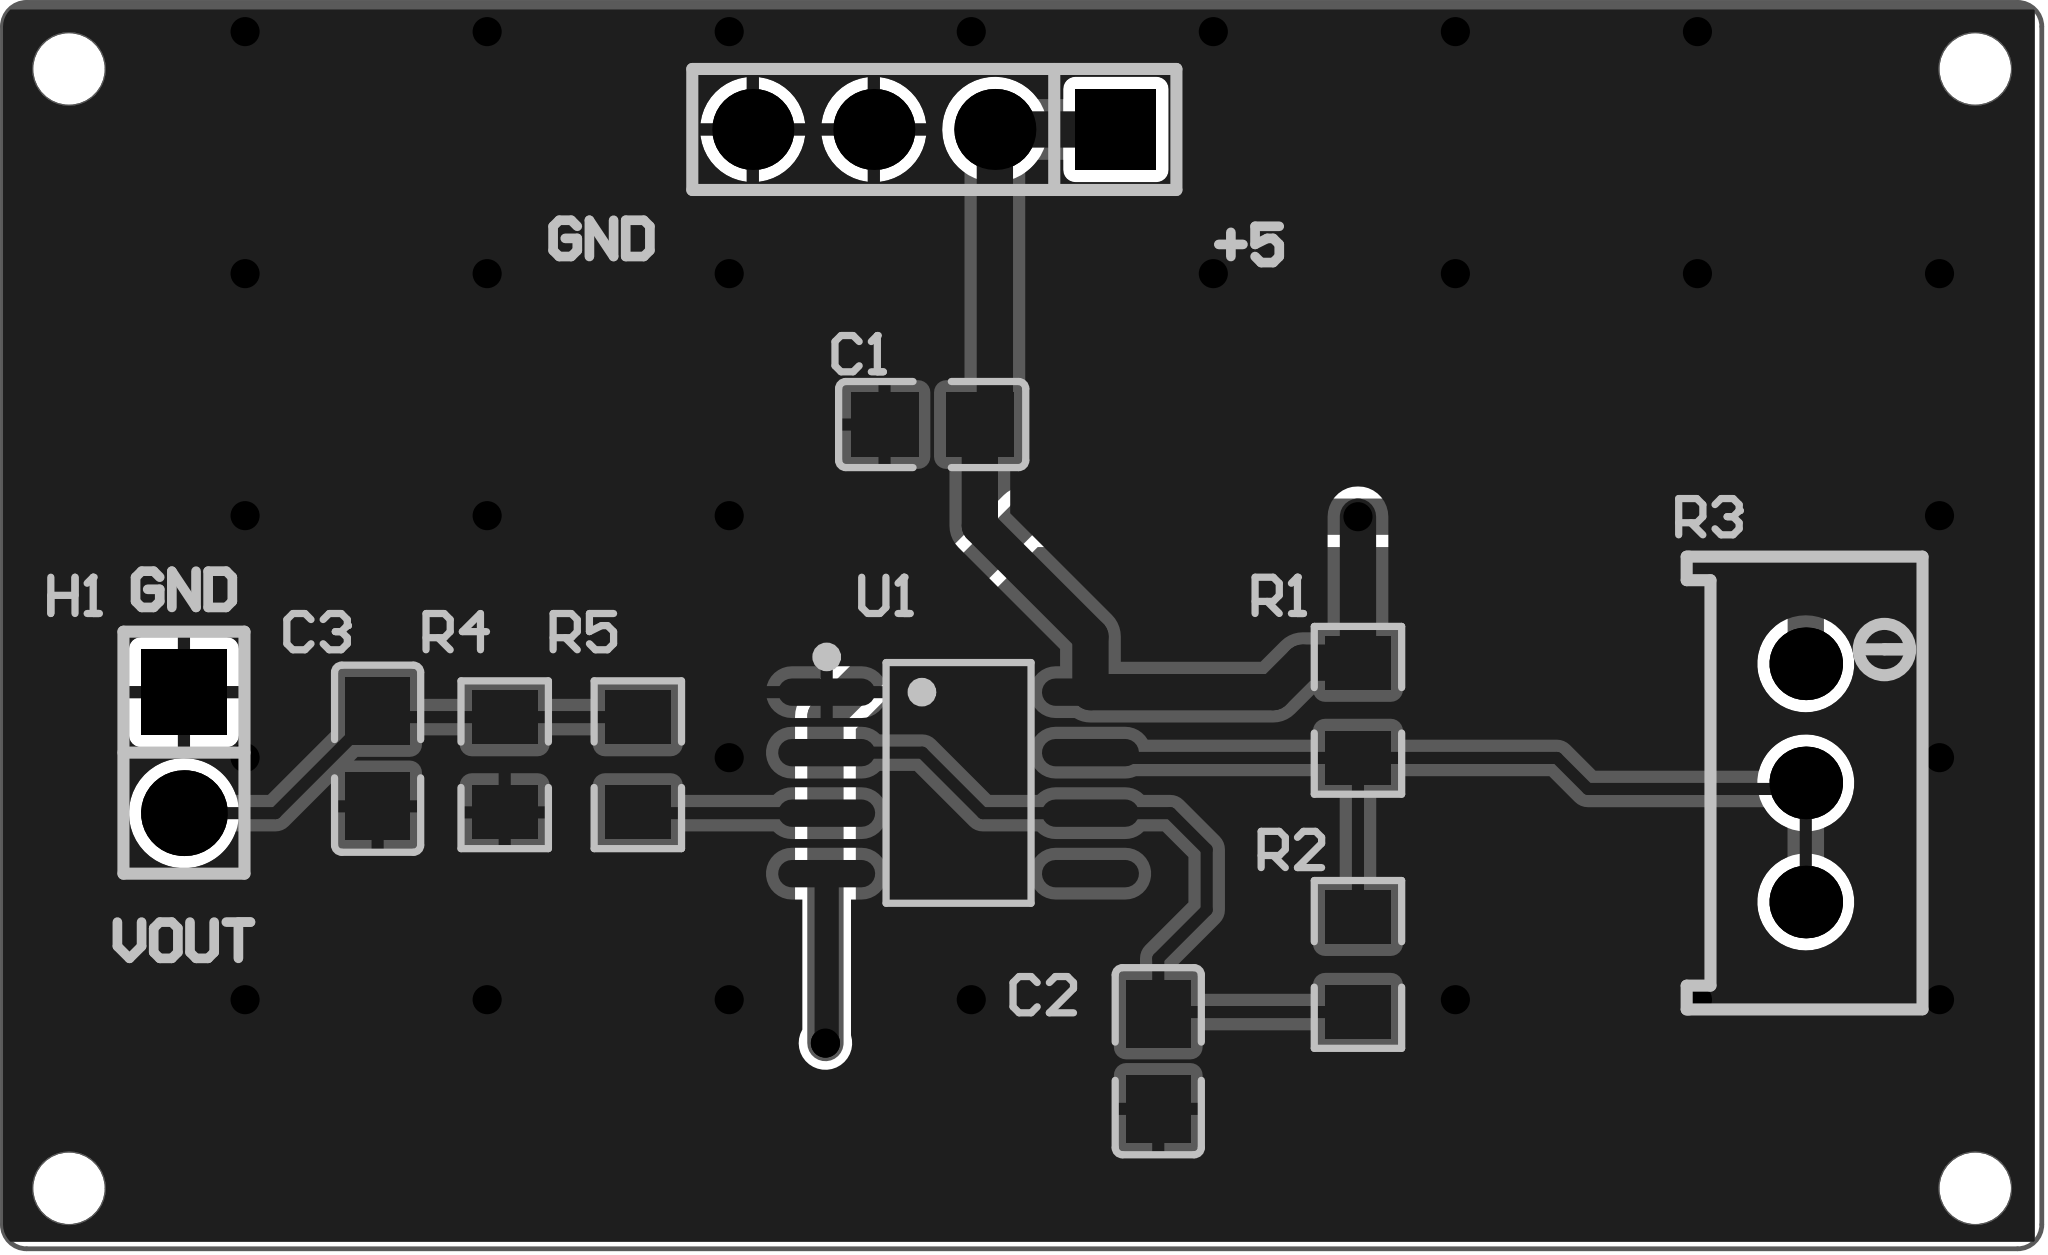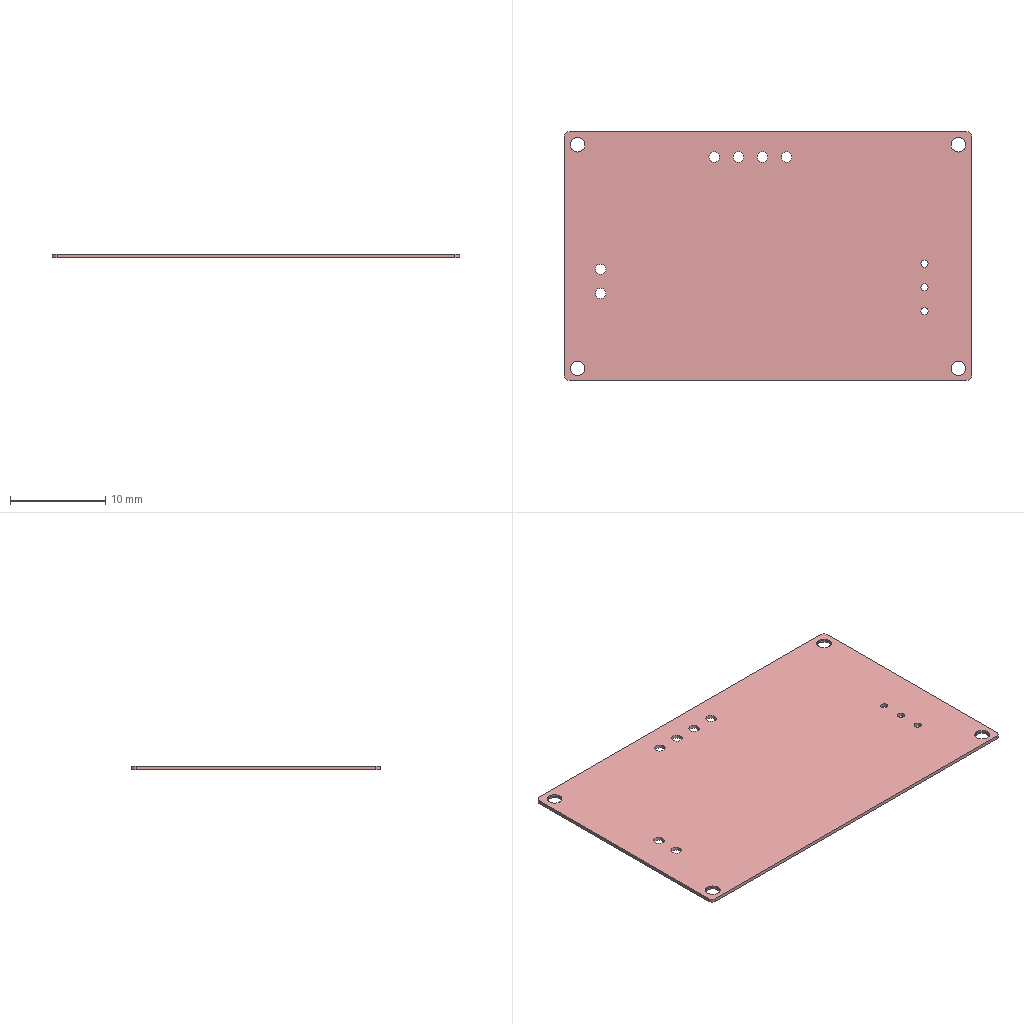Circuit board layout | Altium Designer | box 42.8 x 26.2 x 0.4 mm
Layer stack:
# Altium Designer layer stack of  (unit mm; dielectric type: 0 none, 1 core, 2 prepreg, 3 surface material)
index,name,kind,layer,copper_thickness_mm,dielectric_type,dielectric_thickness_mm,dielectric_material,dielectric_constant
0,Top Paste Mask Layer,other,,,,,,
1,Top Silkscreen Layer,other,,,,,,
2,Top Solder Mask Layer,dielectric,,,3,0.01,,3.3
3,Top Layer,copper,Top Layer,0,,,,
4,SUBSTRATE1,dielectric,,,3,0.32,FR-4,4.8
5,Bottom Layer,copper,Bottom Layer,0.035,,,,
6,Bottom Solder Mask Layer,dielectric,,,3,0.01,,3.3
7,Bottom Silkscreen Layer,other,,,,,,
8,Bottom Paste Mask Layer,other,,,,,,
# drill layer pairs: low layer,high layer
drill_pair,Top Layer,Bottom Layer
Part placement:
Designator,Comment,Layer,Footprint,Center-X(mm),Center-Y(mm),Rotation
C1,1uF,TopLayer,C0805,95.713,93.501,0
C2,10nF,TopLayer,C0805,100.457,80.137,90
CN1,A2541WV-4P,TopLayer,HDR-TH_4P-P2.54-V-M,95.758,99.695,180
H1,A2541WV-2P,TopLayer,HDR-TH_P2.54-H-M_A2541WV-2P,80.01,86.614,270
R1,5kO,TopLayer,R0805,104.648,87.503,90
R2,3kO,TopLayer,R0805,104.648,82.169,90
R3,5kO,TopLayer,RES-ADJ-TH_3P-L10.0-W10.0-P2.50-L,114.046,85.979,270
U1,100kHz,TopLayer,SOP-8_L5.0-W4.0-P1.27-LS6.0-BL,96.266,85.979,270
C3,200pF,TopLayer,C0805,84.074,86.487,90
R4,10kO,TopLayer,R0805,86.741,86.36,90
R5,10kO,TopLayer,R0805,89.535,86.36,270
Pad and via stacks:
# Altium Designer via and pad stacks of  (unit mm). Each distinct definition once, with the count of objects using it.
# via: kind,start_layer,end_layer,hole_mm,diameter_mm,mode(0 simple;1 top-mid-bottom;2 full stack),diameter_per_layer,count,example_net
# pad: kind,layer,hole_mm,hole_type(0 round;1 square;2 slot),plating,top_size,top_shape(1 round;2 rect;3 octagon;9 rounded rect),mid_size,bottom_size,mode,footprint,size_per_layer,count,example
pad,Top Layer,0,0,plated,1.41x1.35,2,1.41x1.35,1.41x1.35,0,C0805,,6,C1.2
pad,Top Layer,0,0,plated,1.133x1.377,2,1.133x1.377,1.133x1.377,0,R0805,,8,R1.2
pad,Top Layer,0,0,plated,0.574x2.035,1,0.574x2.035,0.574x2.035,0,SOP-8_L5.0-W4.0-P1.27-LS6.0-BL,,8,U1.1
pad,Multi-Layer,1.1,0,plated,1.7x1.7,2,1.7x1.7,1.7x1.7,0,HDR-TH_4P-P2.54-V-M,,1,CN1.1
pad,Multi-Layer,1.1,0,plated,1.7x1.7,1,1.7x1.7,1.7x1.7,0,HDR-TH_4P-P2.54-V-M,,3,CN1.2
pad,Multi-Layer,1.1,0,plated,1.8x1.8,2,1.8x1.8,1.8x1.8,0,HDR-TH_P2.54-H-M_A2541WV-2P,,1,H1.1
pad,Multi-Layer,1.1,0,plated,1.8x1.8,1,1.8x1.8,1.8x1.8,0,HDR-TH_P2.54-H-M_A2541WV-2P,,1,H1.2
pad,Multi-Layer,0.762,0,plated,1.524x1.524,1,1.524x1.524,1.524x1.524,0,RES-ADJ-TH_3P-L10.0-W10.0-P2.50-L,,3,R3.2
via,Top Layer,Bottom Layer,0.3048,0.61,0,,30,+5V
Copper pours:
name,layer,net,type(0 solid;1 hatched;2 none)
Top Layer-GND,Top Layer,GND,0
Bottom Layer-GND,Bottom Layer,GND,0
Design rules, without the lines most boards share:
# Altium Designer design rules of  (exported by Altium Designer, unit mm)
# columns: name | kind | enabled | priority | scope1 | scope2 | descriptor | typed fields (field=value)
copperThickness2oz | 0 | disabled | 1 | All | All | Clearance Constraint (Gap=6mil) (Disabled)(All),(All) | gap=0.1524
Plane_innerPlane | 0 | disabled | 2 | All | All | Clearance Constraint (Gap=6mil) (Disabled)(All),(All) | gap=0.1524
Copper_copperRegion | 0 | disabled | 3 | All | All | Clearance Constraint (Gap=6mil) (Disabled)(All),(All) | gap=0.1524
copperThickness1oz | 0 | enabled | 4 | All | All | Clearance Constraint (Gap=6mil) (All),(All) | gap=0.1524
differentialPair | 51 | enabled | 1 | All | All | Differential Pairs Uncoupled Length using the Gap Constraints (Min=99999mil) (Max=6mil) (Prefered=6mil)  and Width Constraints (Min=5mil) (Max=100mil) (Prefered=10mil) (All) |
solderMaskExpansion | 13 | enabled | 1 | All | All | Solder Mask Expansion (Expansion =2mil) (All) | expansion=0.0508